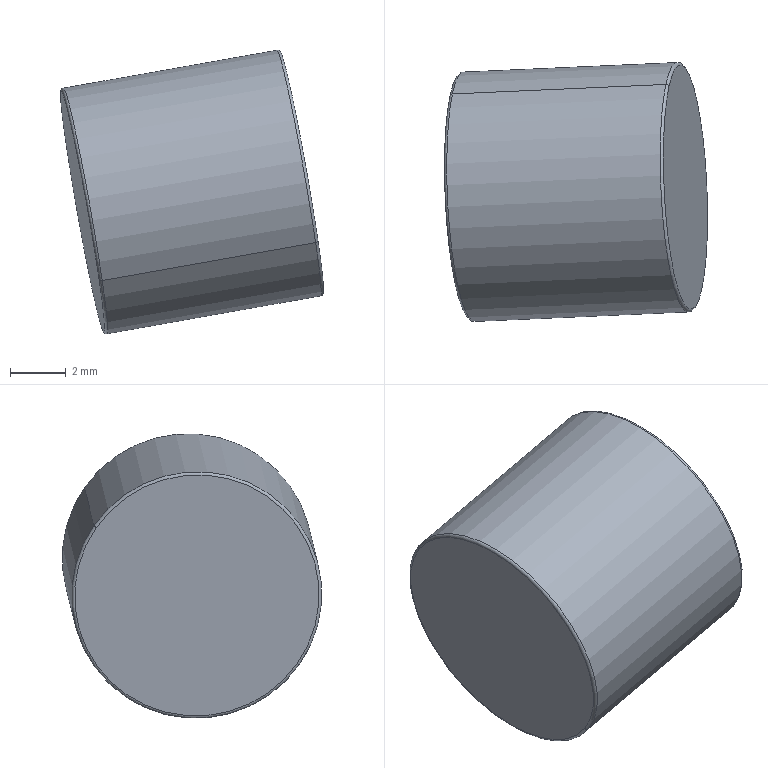Part | SolidWorks | features BaseBody 1 | 1 solid | 8 faces | box 9.458 x 9.331 x 10.228 mm | volume 508.817 mm3 | torus 4 | cylinder 2 | plane 2 | commonest cylinder face diameters 9 x2
STEP:
#1=CARTESIAN_POINT('',(257.363,10.331,29.201));
#2=VERTEX_POINT('',#1);
#3=CARTESIAN_POINT('',(258.578,2.949,24.199));
#4=VERTEX_POINT('',#3);
#5=CARTESIAN_POINT('',(257.971,6.64,26.7));
#6=DIRECTION('',(-0.9836,-0.04348,-0.1748));
#7=DIRECTION('',(0.135,-0.8203,-0.5558));
#8=AXIS2_PLACEMENT_3D('',#5,#6,#7);
#9=CIRCLE('',#8,4.5);
#10=EDGE_CURVE('',#2,#4,#9,.T.);
#11=ORIENTED_EDGE('',*,*,#10,.F.);
#12=CARTESIAN_POINT('',(257.475,10.254,29.163));
#13=VERTEX_POINT('',#12);
#14=CARTESIAN_POINT('',(257.377,10.249,29.146));
#15=DIRECTION('',(0.1192,0.5703,-0.8127));
#16=DIRECTION('',(0.,0.8186,0.5744));
#17=AXIS2_PLACEMENT_3D('',#14,#15,#16);
#18=CIRCLE('',#17,0.1);
#19=EDGE_CURVE('',#2,#13,#18,.T.);
#20=ORIENTED_EDGE('',*,*,#19,.T.);
#21=CARTESIAN_POINT('',(258.663,3.035,24.272));
#22=VERTEX_POINT('',#21);
#23=CARTESIAN_POINT('',(258.069,6.645,26.718));
#24=DIRECTION('',(0.9836,0.04348,0.1748));
#25=DIRECTION('',(0.135,-0.8203,-0.5558));
#26=AXIS2_PLACEMENT_3D('',#23,#24,#25);
#27=CIRCLE('',#26,4.4);
#28=EDGE_CURVE('',#22,#13,#27,.T.);
#29=ORIENTED_EDGE('',*,*,#28,.F.);
#30=CARTESIAN_POINT('',(258.565,3.031,24.255));
#31=DIRECTION('',(-0.1192,-0.5703,0.8127));
#32=DIRECTION('',(0.,-0.8186,-0.5744));
#33=AXIS2_PLACEMENT_3D('',#30,#31,#32);
#34=CIRCLE('',#33,0.1);
#35=EDGE_CURVE('',#4,#22,#34,.T.);
#36=ORIENTED_EDGE('',*,*,#35,.F.);
#37=EDGE_LOOP('',(#11,#20,#29,#36));
#38=FACE_OUTER_BOUND('',#37,.T.);
#39=CARTESIAN_POINT('',(257.971,6.64,26.7));
#40=DIRECTION('',(0.9836,0.04348,0.1748));
#41=DIRECTION('',(0.135,-0.8203,-0.5558));
#42=AXIS2_PLACEMENT_3D('',#39,#40,#41);
#43=TOROIDAL_SURFACE('',#42,4.4,0.1);
#44=ADVANCED_FACE('',(#38),#43,.T.);
#45=CARTESIAN_POINT('',(249.606,9.906,27.765));
#46=VERTEX_POINT('',#45);
#47=CARTESIAN_POINT('',(250.794,2.687,22.874));
#48=VERTEX_POINT('',#47);
#49=CARTESIAN_POINT('',(250.2,6.297,25.319));
#50=DIRECTION('',(-0.9836,-0.04348,-0.1748));
#51=DIRECTION('',(0.135,-0.8203,-0.5558));
#52=AXIS2_PLACEMENT_3D('',#49,#50,#51);
#53=CIRCLE('',#52,4.4);
#54=EDGE_CURVE('',#46,#48,#53,.T.);
#55=ORIENTED_EDGE('',*,*,#54,.F.);
#56=CARTESIAN_POINT('',(249.691,9.992,27.838));
#57=VERTEX_POINT('',#56);
#58=CARTESIAN_POINT('',(249.704,9.91,27.782));
#59=DIRECTION('',(0.1192,0.5703,-0.8127));
#60=DIRECTION('',(0.,0.8186,0.5744));
#61=AXIS2_PLACEMENT_3D('',#58,#59,#60);
#62=CIRCLE('',#61,0.1);
#63=EDGE_CURVE('',#46,#57,#62,.T.);
#64=ORIENTED_EDGE('',*,*,#63,.T.);
#65=CARTESIAN_POINT('',(250.906,2.61,22.836));
#66=VERTEX_POINT('',#65);
#67=CARTESIAN_POINT('',(250.298,6.301,25.337));
#68=DIRECTION('',(0.9836,0.04348,0.1748));
#69=DIRECTION('',(0.135,-0.8203,-0.5558));
#70=AXIS2_PLACEMENT_3D('',#67,#68,#69);
#71=CIRCLE('',#70,4.5);
#72=EDGE_CURVE('',#66,#57,#71,.T.);
#73=ORIENTED_EDGE('',*,*,#72,.F.);
#74=CARTESIAN_POINT('',(250.893,2.692,22.891));
#75=DIRECTION('',(-0.1192,-0.5703,0.8127));
#76=DIRECTION('',(0.,-0.8186,-0.5744));
#77=AXIS2_PLACEMENT_3D('',#74,#75,#76);
#78=CIRCLE('',#77,0.1);
#79=EDGE_CURVE('',#48,#66,#78,.T.);
#80=ORIENTED_EDGE('',*,*,#79,.F.);
#81=EDGE_LOOP('',(#55,#64,#73,#80));
#82=FACE_OUTER_BOUND('',#81,.T.);
#83=CARTESIAN_POINT('',(250.298,6.301,25.337));
#84=DIRECTION('',(0.9836,0.04348,0.1748));
#85=DIRECTION('',(0.135,-0.8203,-0.5558));
#86=AXIS2_PLACEMENT_3D('',#83,#84,#85);
#87=TOROIDAL_SURFACE('',#86,4.4,0.1);
#88=ADVANCED_FACE('',(#82),#87,.T.);
#89=ORIENTED_EDGE('',*,*,#10,.T.);
#90=CARTESIAN_POINT('',(258.677,2.953,24.217));
#91=DIRECTION('',(-0.9836,-0.04348,-0.1748));
#92=VECTOR('',#91,1000.);
#93=LINE('',#90,#92);
#94=EDGE_CURVE('',#4,#66,#93,.T.);
#95=ORIENTED_EDGE('',*,*,#94,.T.);
#96=ORIENTED_EDGE('',*,*,#72,.T.);
#97=CARTESIAN_POINT('',(257.461,10.336,29.219));
#98=DIRECTION('',(-0.9836,-0.04348,-0.1748));
#99=VECTOR('',#98,1000.);
#100=LINE('',#97,#99);
#101=EDGE_CURVE('',#2,#57,#100,.T.);
#102=ORIENTED_EDGE('',*,*,#101,.F.);
#103=EDGE_LOOP('',(#89,#95,#96,#102));
#104=FACE_OUTER_BOUND('',#103,.T.);
#105=CARTESIAN_POINT('',(258.069,6.645,26.718));
#106=DIRECTION('',(-0.9836,-0.04348,-0.1748));
#107=DIRECTION('',(-0.135,0.8203,0.5558));
#108=AXIS2_PLACEMENT_3D('',#105,#106,#107);
#109=CYLINDRICAL_SURFACE('',#108,4.5);
#110=ADVANCED_FACE('',(#104),#109,.T.);
#111=ORIENTED_EDGE('',*,*,#94,.F.);
#112=CARTESIAN_POINT('',(257.971,6.64,26.7));
#113=DIRECTION('',(-0.9836,-0.04348,-0.1748));
#114=DIRECTION('',(0.135,-0.8203,-0.5558));
#115=AXIS2_PLACEMENT_3D('',#112,#113,#114);
#116=CIRCLE('',#115,4.5);
#117=EDGE_CURVE('',#4,#2,#116,.T.);
#118=ORIENTED_EDGE('',*,*,#117,.T.);
#119=ORIENTED_EDGE('',*,*,#101,.T.);
#120=CARTESIAN_POINT('',(250.298,6.301,25.337));
#121=DIRECTION('',(0.9836,0.04348,0.1748));
#122=DIRECTION('',(0.135,-0.8203,-0.5558));
#123=AXIS2_PLACEMENT_3D('',#120,#121,#122);
#124=CIRCLE('',#123,4.5);
#125=EDGE_CURVE('',#57,#66,#124,.T.);
#126=ORIENTED_EDGE('',*,*,#125,.T.);
#127=EDGE_LOOP('',(#111,#118,#119,#126));
#128=FACE_OUTER_BOUND('',#127,.T.);
#129=CARTESIAN_POINT('',(258.069,6.645,26.718));
#130=DIRECTION('',(-0.9836,-0.04348,-0.1748));
#131=DIRECTION('',(-0.135,0.8203,0.5558));
#132=AXIS2_PLACEMENT_3D('',#129,#130,#131);
#133=CYLINDRICAL_SURFACE('',#132,4.5);
#134=ADVANCED_FACE('',(#128),#133,.T.);
#135=ORIENTED_EDGE('',*,*,#28,.T.);
#136=CARTESIAN_POINT('',(258.069,6.645,26.718));
#137=DIRECTION('',(0.9836,0.04348,0.1748));
#138=DIRECTION('',(0.135,-0.8203,-0.5558));
#139=AXIS2_PLACEMENT_3D('',#136,#137,#138);
#140=CIRCLE('',#139,4.4);
#141=EDGE_CURVE('',#13,#22,#140,.T.);
#142=ORIENTED_EDGE('',*,*,#141,.T.);
#143=EDGE_LOOP('',(#135,#142));
#144=FACE_OUTER_BOUND('',#143,.T.);
#145=CARTESIAN_POINT('',(258.069,6.645,26.718));
#146=DIRECTION('',(0.9836,0.04348,0.1748));
#147=DIRECTION('',(0.135,-0.8203,-0.5558));
#148=AXIS2_PLACEMENT_3D('',#145,#146,#147);
#149=PLANE('',#148);
#150=ADVANCED_FACE('',(#144),#149,.T.);
#151=CARTESIAN_POINT('',(250.2,6.297,25.319));
#152=DIRECTION('',(-0.9836,-0.04348,-0.1748));
#153=DIRECTION('',(0.135,-0.8203,-0.5558));
#154=AXIS2_PLACEMENT_3D('',#151,#152,#153);
#155=CIRCLE('',#154,4.4);
#156=EDGE_CURVE('',#48,#46,#155,.T.);
#157=ORIENTED_EDGE('',*,*,#156,.T.);
#158=ORIENTED_EDGE('',*,*,#54,.T.);
#159=EDGE_LOOP('',(#157,#158));
#160=FACE_OUTER_BOUND('',#159,.T.);
#161=CARTESIAN_POINT('',(250.2,6.297,25.319));
#162=DIRECTION('',(0.9836,0.04348,0.1748));
#163=DIRECTION('',(0.135,-0.8203,-0.5558));
#164=AXIS2_PLACEMENT_3D('',#161,#162,#163);
#165=PLANE('',#164);
#166=ADVANCED_FACE('',(#160),#165,.F.);
#167=ORIENTED_EDGE('',*,*,#63,.F.);
#168=ORIENTED_EDGE('',*,*,#156,.F.);
#169=ORIENTED_EDGE('',*,*,#79,.T.);
#170=ORIENTED_EDGE('',*,*,#125,.F.);
#171=EDGE_LOOP('',(#167,#168,#169,#170));
#172=FACE_OUTER_BOUND('',#171,.T.);
#173=CARTESIAN_POINT('',(250.298,6.301,25.337));
#174=DIRECTION('',(0.9836,0.04348,0.1748));
#175=DIRECTION('',(0.135,-0.8203,-0.5558));
#176=AXIS2_PLACEMENT_3D('',#173,#174,#175);
#177=TOROIDAL_SURFACE('',#176,4.4,0.1);
#178=ADVANCED_FACE('',(#172),#177,.T.);
#179=ORIENTED_EDGE('',*,*,#19,.F.);
#180=ORIENTED_EDGE('',*,*,#117,.F.);
#181=ORIENTED_EDGE('',*,*,#35,.T.);
#182=ORIENTED_EDGE('',*,*,#141,.F.);
#183=EDGE_LOOP('',(#179,#180,#181,#182));
#184=FACE_OUTER_BOUND('',#183,.T.);
#185=CARTESIAN_POINT('',(257.971,6.64,26.7));
#186=DIRECTION('',(0.9836,0.04348,0.1748));
#187=DIRECTION('',(0.135,-0.8203,-0.5558));
#188=AXIS2_PLACEMENT_3D('',#185,#186,#187);
#189=TOROIDAL_SURFACE('',#188,4.4,0.1);
#190=ADVANCED_FACE('',(#184),#189,.T.);
#191=CLOSED_SHELL('',(#44,#88,#110,#134,#150,#166,#178,#190));
#192=MANIFOLD_SOLID_BREP('',#191);
#193=CARTESIAN_POINT('',(0.,0.,0.));
#194=DIRECTION('',(0.,0.,1.));
#195=DIRECTION('',(1.,0.,0.));
#196=AXIS2_PLACEMENT_3D('',#193,#194,#195);
#197=(LENGTH_UNIT()NAMED_UNIT(*)SI_UNIT(.MILLI.,.METRE.));
#198=UNCERTAINTY_MEASURE_WITH_UNIT(LENGTH_MEASURE(0.00001),#197,'','');
#199=(NAMED_UNIT(*)PLANE_ANGLE_UNIT()SI_UNIT($,.RADIAN.));
#200=(NAMED_UNIT(*)SI_UNIT($,.STERADIAN.)SOLID_ANGLE_UNIT());
#201=(GEOMETRIC_REPRESENTATION_CONTEXT(3)GLOBAL_UNCERTAINTY_ASSIGNED_CONTEXT((#198))GLOBAL_UNIT_ASSIGNED_CONTEXT((#197,#199,#200))REPRESENTATION_CONTEXT('',''));
#202=ADVANCED_BREP_SHAPE_REPRESENTATION('',(#192,#196),#201);